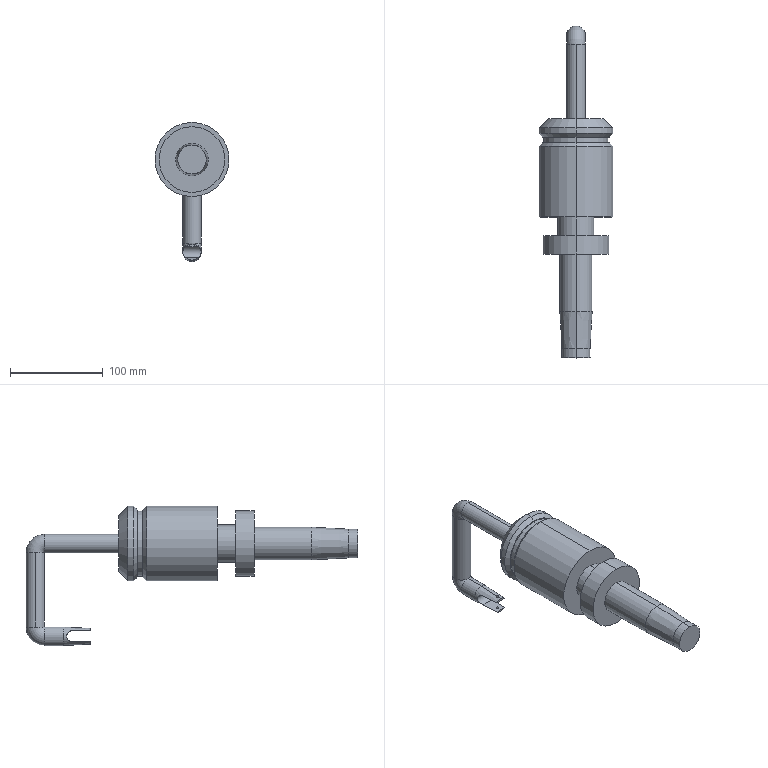Part | SolidWorks | features ICE 10, Chamfer 3, Extrusion 1, RefAxis 1, Revolution 1, Sweep 1 | 1 solid | 48 faces | box 80 x 358 x 150 mm | volume 786252 mm3 | cylinder 25 | plane 11 | cone 10 | torus 2 | commonest cylinder face diameters 20 x6 3 x4 80 x4 31 x2 35.193 x2 40 x2